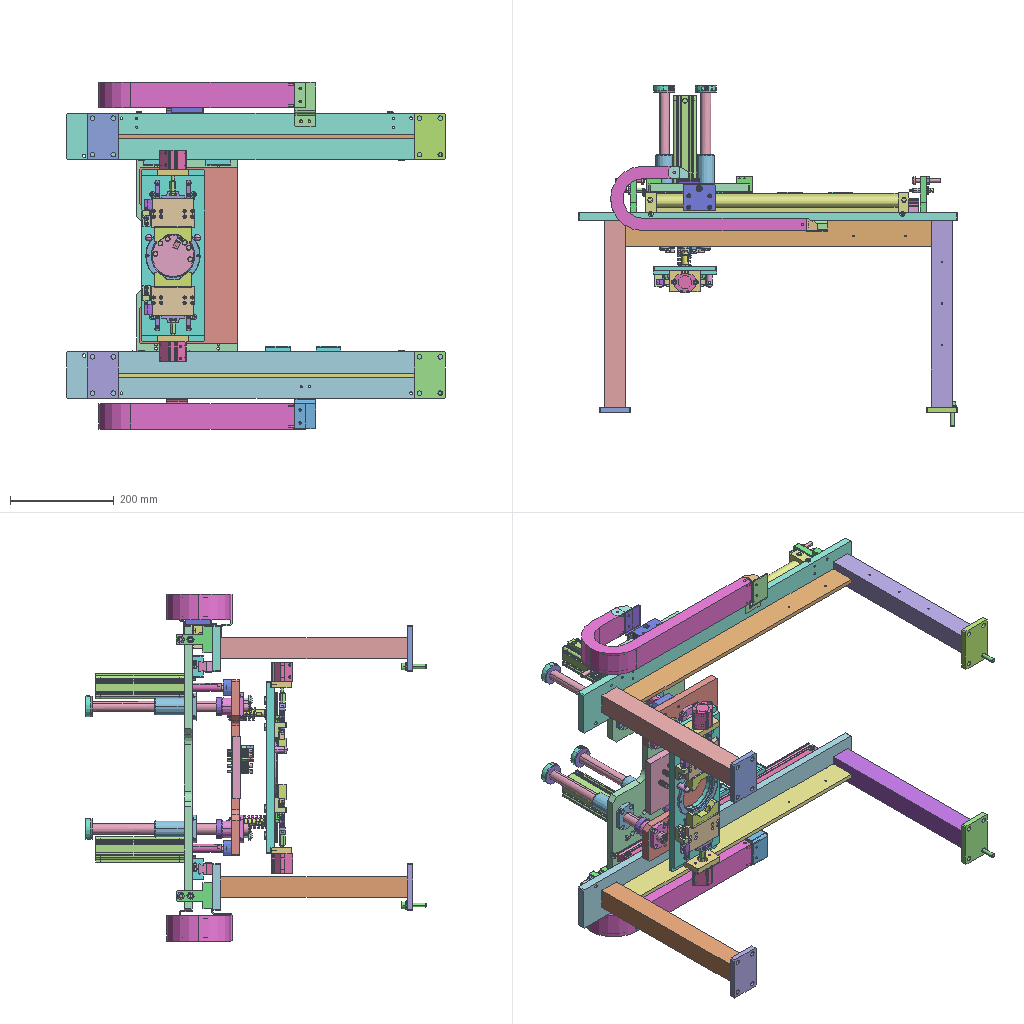Assembly | STEP file | 84 different items | 191 placed | box 730 x 656 x 669 mm
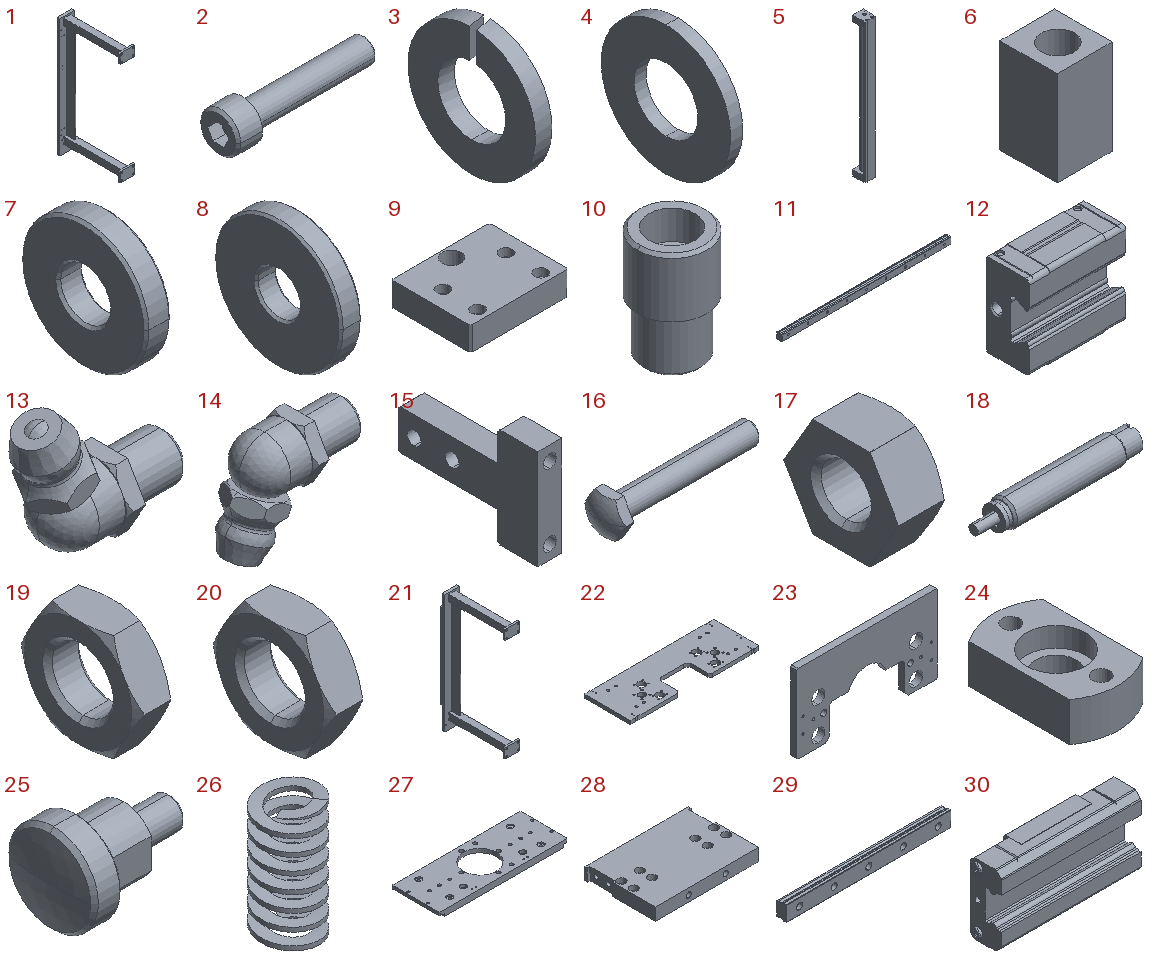Parts list (item | name | quantity | parent item | size | volume):
1 | 227H056235 BKT L_Default | x1 | in BKE LEFT ASSY_Default | 90 x 397 x 730 mm | 1763057 mm3
2 | CB8-40_Default | x2 | in CB8-40_SW8_W8_Default | 48 x 13 x 13 mm | 2919 mm3
3 | SW8_Default | x2 | in CB8-40_SW8_W8_Default | 2 x 15.4 x 15.396 mm | 260.908 mm3
4 | W8_Default | x2 | in CB8-40_SW8_W8_Default | 1.6 x 17 x 17 mm | 274.5 mm3
5 | 1_22 | x1 | in CY3R20-400_0_0_0_ | 38 x 45 x 507 mm | 342887 mm3
6 | 2_22 | x1 | in CY3R20-400_0_0_0_ | 36 x 37.5 x 62 mm | 60624 mm3
7 | wasmh10_4_2_2_03 | x2 | in BKE LEFT ASSY_Default | 2 x 10 x 10 mm | 130.188 mm3
8 | wasmh12_4_2_2_03 | x4 | in BKE LEFT ASSY_Default, BKE Right ASSY_Default | 2 x 12 x 12 mm | 199.051 mm3
9 | 227H056245 Move Block_Default | x1 | in BKE LEFT ASSY_Default | 62 x 50 x 15 mm | 43132 mm3
10 | 227H056246 Shaft_Default | x1 | in BKE LEFT ASSY_Default | 12 x 12 x 19 mm | 1355 mm3
11 | SSR20XV52020 Track | x2 | in SSR20XV2UU520200B047_700 | 520 x 15.5 x 20 mm | 137719 mm3
12 | SSR20XVUUB Slide15-25 | x4 | in SSR20XV2UU520200B047_700 | 47.7 x 22 x 42 mm | 34844 mm3
13 | SSR20XVUUBGNPJ-20-25 | x2 | in SSR20XV2UU520200B047_700 | 18.6 x 9.238 x 15.618 mm | 860 mm3
14 | SSR20XVUUBGNPJ2-20-25 | x2 | in SSR20XV2UU520200B047_700 | 18.6 x 9.238 x 15.618 mm | 860.005 mm3
15 | 227H056256 Stop Block_Default | x5 | in TRU, P_Default | 12 x 70 x 50 mm | 21777 mm3
16 | 1_12 | x5 | in stbb8_50_2_03 | - | 3160 mm3
17 | 2_12 | x5 | in stbb8_50_2_03 | 6.5 x 15 x 13 mm | 713.15 mm3
18 | Sceond1_16 | x5 | in SceondRB0806_0_ | 46.8 x 8 x 8 mm | 1959 mm3
19 | Sceond2_16 | x5 | in SceondRB0806_0_ | 4 x 13.856 x 12 mm | 338.014 mm3
20 | Sceond3_11 | x5 | in SceondRB0806_0_ | 4 x 13.856 x 12 mm | 338.014 mm3
21 | 227H056236 BKT R_Default | x1 | in BKE Right ASSY_Default | 90 x 397 x 730 mm | 1763979 mm3
22 | 227H056239 Base | x1 | in qnBANSONG_Default | 550 x 195 x 15 mm | 1337407 mm3
23 | 227H056238 Middle Base_Default | x1 | in qnBANSONG_Default | 340 x 15 x 190 mm | 662186 mm3
24 | qnSceondFJMC8part4 | x2 | in qnSceondFJMC8-00_FJMC8 | 30 x 51 x 16 mm | 15639 mm3
25 | qnSceondFJMC8part5 | x2 | in qnSceondFJMC8-00_FJMC8 | 32 x 23 x 23 mm | 5961 mm3
26 | SWY24.5-55_Default | x2 | in qnBANSONG_Default | 26.648 x 26.648 x 55 mm | 5041 mm3
27 | 227H056237 Under Base | x1 | in qnSceondMove 1_Default | 332 x 122 x 15 mm | 468693 mm3
28 | 227H056248 JIG Block | x2 | in qnSceondMove 1_Default | 84 x 57 x 10 mm | 44690 mm3
29 | 2SRS9MUU+95L | x4 | in 29 | 95 x 5.5 x 9 mm | 3697 mm3
30 | qnSceond_SRS9MQZUU Slider | x4 | in 29 | 40.8 x 9.1 x 20 mm | 5179 mm3
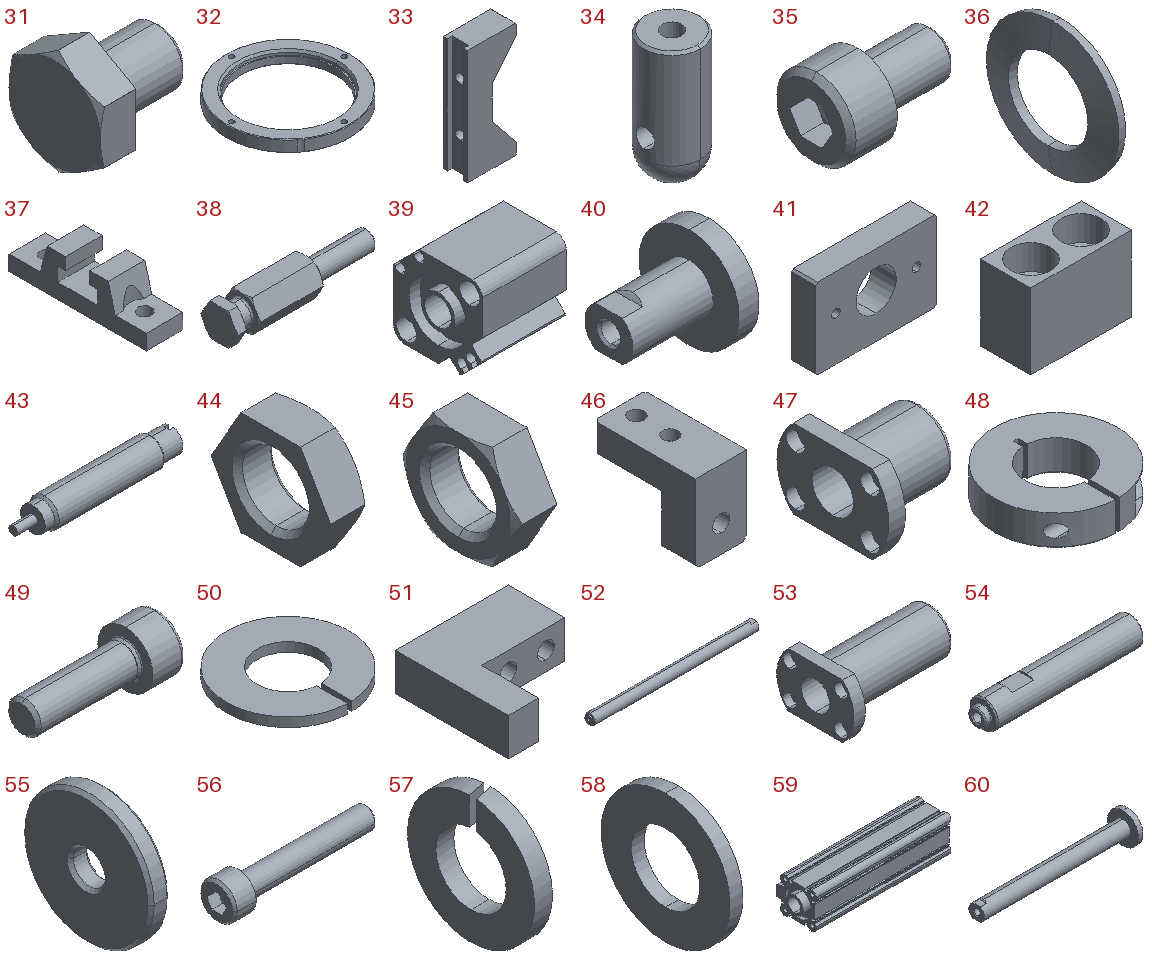31 | STEHN13 | x4 | in qnSceondMove 1_Default | 15 x 13 x 15 mm | 1216 mm3
32 | 227H056250 JIG_Default | x1 | in qnSceondMove 1_Default | 105 x 105 x 10 mm | 33679 mm3
33 | 227H056247 JIG_Default | x2 | in qnSceondMove 1_Default | 30 x 15 x 70 mm | 19012 mm3
34 | 227H056251 Pin_Default | x2 | in qnSceondMove 1_Default | 12 x 12 x 27 mm | 2502 mm3
35 | CB5-8_Default | x1 | in CB5-8_CW5_Default | 13 x 8.5 x 8.5 mm | 398.056 mm3
36 | CW5_Default | x1 | in CB5-8_CW5_Default | 0.85 x 9 x 9 mm | 22.263 mm3
37 | hlre7_2_03 | x2 | in qnSceondMove 1_Default | 12 x 45 x 13.5 mm | 3705 mm3
38 | fjdl6_1_0_4_20_2_03 | x2 | in qnSceondMove 1_Default | 46 x 11.547 x 10 mm | 2689 mm3
39 | 1_9 | x2 | in CDQ2B25-5DZ_0_0_0_ | 37.5 x 40 x 40 mm | 38658 mm3
40 | 2_9 | x2 | in CDQ2B25-5DZ_0_0_0_ | 25 x 25 x 25 mm | 4428 mm3
41 | 227H056249 Cylinder BKT_Default | x2 | in qnSceondMove 1_Default | 60 x 12 x 40 mm | 24374 mm3
42 | 227H056259 Stop Block_Default | x2 | in qnSceondMove 1_Default | 20 x 10 x 15 mm | 2179 mm3
43 | 1_10 | x2 | in RB0604_0_ | 32.5 x 6 x 6 mm | 755.606 mm3
44 | 2_10 | x2 | in RB0604_0_ | 3 x 9.238 x 8 mm | 99.469 mm3
45 | 3_1 | x2 | in RB0604_0_ | 3 x 9.238 x 8 mm | 99.469 mm3
46 | 227H056261 Stop Block_Default | x2 | in qnSceondMove 1_Default | 15 x 30 x 23 mm | 5038 mm3
47 | qnslhfc20_2_03 | x4 | in qnBANSONG_Default | 42 x 54 x 38 mm | 27385 mm3
48 | qnSceond1_10 | x4 | in qnSceondpscdj20_13_2_031 | 40 x 39.986 x 10 mm | 8415 mm3
49 | qnSceond2_10 | x4 | in qnSceondpscdj20_13_2_031 | 21 x 8.5 x 8.5 mm | 547.959 mm3
50 | qnSceond3_2 | x4 | in qnSceondpscdj20_13_2_031 | 40 x 39.986 x 3 mm | 2782 mm3
51 | 227H056244 Stopper_Default | x4 | in qnBANSONG_Default | 30 x 30 x 10 mm | 4879 mm3
52 | sfpg20_315_f3_p15_m6_sc305_2_03 | x4 | in qnBANSONG_Default | 318 x 20 x 20 mm | 98846 mm3
53 | lhfcwmf20_2_03 | x4 | in qnBANSONG_Default | 80 x 54 x 38 mm | 46009 mm3
54 | sfppa13_68_f3_p8_m5_n5_sc10_2_03 | x2 | in qnBANSONG_Default | 71 x 13 x 13 mm | 8114 mm3
55 | wssb20_5_3_2_03 | x2 | in qnBANSONG_Default | 3 x 20 x 20 mm | 863.938 mm3
56 | CB5-30_Default | x1 | in CB5-30_SW5_W5_Default | 35 x 8.5 x 8.5 mm | 830.025 mm3
57 | SW5_Default | x1 | in CB5-30_SW5_W5_Default | 1.3 x 9.2 x 9.198 mm | 58.481 mm3
58 | W5_Default | x1 | in CB5-30_SW5_W5_Default | 1 x 10 x 10 mm | 56.478 mm3
59 | 1 | x2 | in CDQ2A32-125DCZ | 175.5 x 49.5 x 45 mm | 171932 mm3
60 | 2 | x2 | in CDQ2A32-125DCZ | 157 x 32 x 32 mm | 34054 mm3
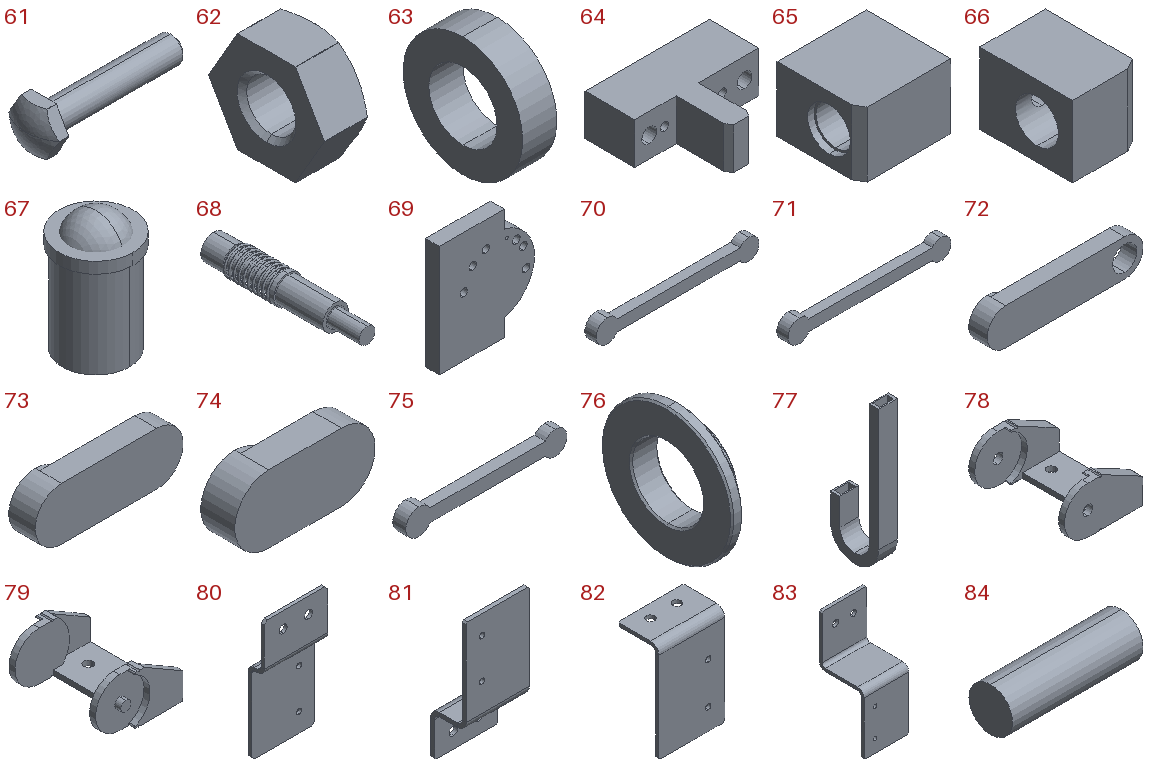61 | 1_5 | x2 | in stbb10_50_2_03 | - | 5335 mm3
62 | 2_5 | x2 | in stbb10_50_2_03 | 8 x 19.6 x 17 mm | 1538 mm3
63 | urws35_20_10_2_03 | x4 | in qnBANSONG_Default | 10 x 35 x 35 mm | 6480 mm3
64 | 22DDSceond144_Default | x1 | in 22DDSceondchatou_Default | 30 x 25 x 10 mm | 3740 mm3
65 | 22DDSceond4trr_Default | x1 | in 22DDSceondchatou_Default | 13.8 x 13 x 10 mm | 1356 mm3
66 | 22DDSceondwrwet_Default | x1 | in 22DDSceondchatou_Default | 9.2 x 13 x 10 mm | 888.519 mm3
67 | 22DDSceondZAL02-M6_Default | x2 | in 22DDSceondchatou_Default | 6.6 x 6.6 x 10.6 mm | 325.856 mm3
68 | 22CPMM160_Default | x6 | in 22DDSceoWWnd Terminal Inspection Tip sss_Default | 9.1 x 48.5 x 9.1 mm | 1897 mm3
69 | jjjj_Default | x1 | in 22DDSceoWWnd Terminal Inspection Tip sss_Default | 102.5 x 15 x 120 mm | 138148 mm3
70 | 222_Default | x1 | in 22DDSceoWWnd Terminal Inspection Tip sss_Default | 86.9 x 6 x 12 mm | 3087 mm3
71 | 333_Default | x1 | in 22DDSceoWWnd Terminal Inspection Tip sss_Default | 88.1 x 6 x 12 mm | 3123 mm3
72 | 444_Default | x1 | in 22DDSceoWWnd Terminal Inspection Tip sss_Default | 51 x 6 x 12 mm | 2767 mm3
73 | TYYUTI_Default | x1 | in 22DDSceoWWnd Terminal Inspection Tip sss_Default | 33.7 x 6 x 12 mm | 1981 mm3
74 | JTJTRUYIU_Default | x1 | in 22DDSceoWWnd Terminal Inspection Tip sss_Default | 24.8 x 6 x 12 mm | 1447 mm3
75 | 111_Default | x1 | in 22DDSceoWWnd Terminal Inspection Tip sss_Default | 75 x 6 x 12 mm | 2730 mm3
76 | ftcm_d16_5_h24_v13_0_t2_0_l5_0_2_03 | x4 | in qnBANSONG_Default | 5 x 24 x 24 mm | 869.825 mm3
77 | 18.37.38-18-18.37.12PZ_Default | x2 | in DFGG_Default | 49 x 124 x 377 mm | 276461 mm3
78 | 18_37_1 | x2 | in DFGG_Default | 40.3 x 49 x 24 mm | 8325 mm3
79 | 18_37_3 | x2 | in DFGG_Default | 40.3 x 49 x 24 mm | 7598 mm3
80 | 227H056252 BKT_Default | x1 | in 17 | 40 x 10 x 80 mm | 6705 mm3
81 | 227h056253 BKT_Default | x1 | in 17 | 40 x 22.5 x 85 mm | 9969 mm3
82 | 227H056254 BKT_Default | x1 | in 17 | 40 x 25 x 60 mm | 6386 mm3
83 | 227H056255 BKT_Default | x1 | in 17 | 40 x 40 x 96 mm | 12819 mm3
84 | HP5-15_Default | x4 | in 17 | 15 x 5 x 5 mm | 294.524 mm3
Placements (level | parent | child | x y z in mm | rotation matrix by rows):
1 | 17 | BKE LEFT ASSY_Default | 0.0 -0.0 230.0 | 1 0 0 0 1 0 0 0 1
2 | BKE LEFT ASSY_Default | 227H056235 BKT L_Default | -0.0 -0.0 -0.0 | 0 0 1 0 1 0 -1 0 0
2 | BKE LEFT ASSY_Default | CB8-40_SW8_W8_Default | 20.0 13.6 -35.0 | 0 1 0 -1 0 0 0 0 1
3 | CB8-40_SW8_W8_Default | CB8-40_Default | -0.0 -0.0 -0.0 | 1 0 0 0 1 0 0 0 1
3 | CB8-40_SW8_W8_Default | SW8_Default | 1.0 -0.0 -0.0 | 1 0 0 0 1 0 0 0 1
3 | CB8-40_SW8_W8_Default | W8_Default | 2.8 -0.0 -0.0 | 1 0 0 0 1 0 0 0 1
2 | BKE LEFT ASSY_Default | CY3R20-400_0_0_0_ | -84.5 481.55 68.762 | 0 0 1 1 0 0 0 1 -0
3 | CY3R20-400_0_0_0_ | 1_22 | -75.55 -42.762 -0.0 | 1 0 0 0 1 0 0 0 1
3 | CY3R20-400_0_0_0_ | 2_22 | -75.55 -42.762 -350.0 | 1 0 0 0 1 0 0 0 1
2 | BKE LEFT ASSY_Default | wasmh10_4_2_2_03 | -76.0 382.0 45.0 | 0 -0.9516 -0.3073 0 0.3073 -0.9516 1 0 0
2 | BKE LEFT ASSY_Default | wasmh10_4_2_2_03 | -561.0 382.0 45.0 | 0 -0.9516 -0.3073 0 0.3073 -0.9516 1 0 0
2 | BKE LEFT ASSY_Default | wasmh12_4_2_2_03 | -55.0 394.0 -45.0 | 0 0 1 0 1 0 -1 0 0
2 | BKE LEFT ASSY_Default | wasmh12_4_2_2_03 | -555.0 394.0 -45.0 | 0 0 1 0 1 0 -1 0 0
2 | BKE LEFT ASSY_Default | 227H056245 Move Block_Default | -467.5 414.5 46.0 | 1 0 0 0 1 0 0 0 1
2 | BKE LEFT ASSY_Default | 227H056246 Shaft_Default | -467.5 431.5 39.0 | 1 0 0 0 1 0 0 0 1
2 | BKE LEFT ASSY_Default | SSR20XV2UU520200B047_700 | -545.0 397.0 -35.0 | 1 0 0 0 1 0 0 0 1
3 | SSR20XV2UU520200B047_700 | SSR20XV52020 Track | -0.0 -0.0 -0.0 | 1 0 0 0 1 0 0 0 1
3 | SSR20XV2UU520200B047_700 | SSR20XVUUB Slide15-25 | 17.5 6.0 0.0 | 1 0 0 0 1 0 0 0 1
3 | SSR20XV2UU520200B047_700 | SSR20XVUUBGNPJ-20-25 | 3.85 6.0 -0.0 | 1 0 0 0 1 0 0 0 1
3 | SSR20XV2UU520200B047_700 | SSR20XVUUB Slide15-25 | 137.5 6.0 0.0 | 1 0 0 0 1 0 0 0 1
3 | SSR20XV2UU520200B047_700 | SSR20XVUUBGNPJ2-20-25 | 51.55 6.0 -0.0 | -1 0 0 0 1 0 0 0 -1
2 | BKE LEFT ASSY_Default | TRU;P_Default | -42.0 420.0 17.0 | 1 0 0 0 1 0 0 0 1
3 | TRU;P_Default | 227H056256 Stop Block_Default | -0.0 -0.0 -0.0 | 1 0 0 0 1 0 0 0 1
3 | TRU;P_Default | stbb8_50_2_03 | -9.75 27.0 -0.0 | 1 0 0 0 0.3709 -0.9287 0 0.9287 0.3709
4 | stbb8_50_2_03 | 1_12 | -0.0 -0.0 -0.0 | 1 0 0 0 1 0 0 0 1
4 | stbb8_50_2_03 | 2_12 | -0.0 -0.0 -0.0 | 1 0 0 0 1 0 0 0 1
3 | TRU;P_Default | SceondRB0806_0_ | -15.0 8.0 -0.0 | 1 0 0 0 0.9995 0.03109 0 -0.03109 0.9995
4 | SceondRB0806_0_ | Sceond1_16 | -0.0 -0.0 -0.0 | 1 0 0 0 1 0 0 0 1
4 | SceondRB0806_0_ | Sceond2_16 | -0.0 -0.0 -0.0 | 1 0 0 0 1 0 0 0 1
4 | SceondRB0806_0_ | Sceond3_11 | 4.733 -0.0 -0.0 | 1 0 0 0 1 0 0 0 1
2 | BKE LEFT ASSY_Default | TRU;P_Default | -588.0 420.0 17.0 | -1 0 0 0 1 0 0 0 -1
3 | TRU;P_Default | 227H056256 Stop Block_Default | -0.0 -0.0 -0.0 | 1 0 0 0 1 0 0 0 1
3 | TRU;P_Default | stbb8_50_2_03 | -9.75 27.0 -0.0 | 1 0 0 0 0.3709 -0.9287 0 0.9287 0.3709
4 | stbb8_50_2_03 | 1_12 | -0.0 -0.0 -0.0 | 1 0 0 0 1 0 0 0 1
4 | stbb8_50_2_03 | 2_12 | -0.0 -0.0 -0.0 | 1 0 0 0 1 0 0 0 1
3 | TRU;P_Default | SceondRB0806_0_ | -15.0 8.0 -0.0 | 1 0 0 0 0.9995 0.03109 0 -0.03109 0.9995
4 | SceondRB0806_0_ | Sceond1_16 | -0.0 -0.0 -0.0 | 1 0 0 0 1 0 0 0 1
4 | SceondRB0806_0_ | Sceond2_16 | -0.0 -0.0 -0.0 | 1 0 0 0 1 0 0 0 1
4 | SceondRB0806_0_ | Sceond3_11 | 4.733 -0.0 -0.0 | 1 0 0 0 1 0 0 0 1
1 | 17 | BKE Right ASSY_Default | -0.0 -0.0 -230.0 | 1 0 0 0 1 0 0 0 1
2 | BKE Right ASSY_Default | 227H056236 BKT R_Default | -0.0 -0.0 -0.0 | 0 0 1 0 1 0 -1 0 0
2 | BKE Right ASSY_Default | CB8-40_SW8_W8_Default | 20.0 13.6 -35.0 | 0 1 0 -1 0 0 0 0 1
3 | CB8-40_SW8_W8_Default | CB8-40_Default | -0.0 -0.0 -0.0 | 1 0 0 0 1 0 0 0 1
3 | CB8-40_SW8_W8_Default | SW8_Default | 1.0 -0.0 -0.0 | 1 0 0 0 1 0 0 0 1
3 | CB8-40_SW8_W8_Default | W8_Default | 2.8 -0.0 -0.0 | 1 0 0 0 1 0 0 0 1
2 | BKE Right ASSY_Default | wasmh12_4_2_2_03 | -555.0 394.0 45.0 | 0 -0.9985 0.05496 0 -0.05496 -0.9985 1 0 -0
2 | BKE Right ASSY_Default | wasmh12_4_2_2_03 | -55.0 394.0 47.0 | 0 0 1 0 1 0 -1 0 0
2 | BKE Right ASSY_Default | SSR20XV2UU520200B047_700 | -545.0 397.0 35.0 | 1 0 0 0 1 0 0 0 1
3 | SSR20XV2UU520200B047_700 | SSR20XV52020 Track | -0.0 -0.0 -0.0 | 1 0 0 0 1 0 0 0 1
3 | SSR20XV2UU520200B047_700 | SSR20XVUUB Slide15-25 | 252.546 6.0 -0.0 | 1 0 0 0 1 0 0 0 1
3 | SSR20XV2UU520200B047_700 | SSR20XVUUBGNPJ-20-25 | 3.85 6.0 -0.0 | 1 0 0 0 1 0 0 0 1
3 | SSR20XV2UU520200B047_700 | SSR20XVUUB Slide15-25 | 349.573 6.0 -0.0 | 1 0 0 0 1 0 0 0 1
3 | SSR20XV2UU520200B047_700 | SSR20XVUUBGNPJ2-20-25 | 51.55 6.0 -0.0 | -1 0 0 0 1 0 0 0 -1
2 | BKE Right ASSY_Default | TRU;P_Default | -588.0 420.0 -17.0 | -1 0 0 0 1 0 0 0 -1
3 | TRU;P_Default | 227H056256 Stop Block_Default | -0.0 -0.0 -0.0 | 1 0 0 0 1 0 0 0 1
3 | TRU;P_Default | stbb8_50_2_03 | -9.75 27.0 -0.0 | 1 0 0 0 0.3709 -0.9287 0 0.9287 0.3709
4 | stbb8_50_2_03 | 1_12 | -0.0 -0.0 -0.0 | 1 0 0 0 1 0 0 0 1
4 | stbb8_50_2_03 | 2_12 | -0.0 -0.0 -0.0 | 1 0 0 0 1 0 0 0 1
3 | TRU;P_Default | SceondRB0806_0_ | -15.0 8.0 -0.0 | 1 0 0 0 0.9995 0.03109 0 -0.03109 0.9995
4 | SceondRB0806_0_ | Sceond1_16 | -0.0 -0.0 -0.0 | 1 0 0 0 1 0 0 0 1
4 | SceondRB0806_0_ | Sceond2_16 | -0.0 -0.0 -0.0 | 1 0 0 0 1 0 0 0 1
4 | SceondRB0806_0_ | Sceond3_11 | 4.733 -0.0 -0.0 | 1 0 0 0 1 0 0 0 1
2 | BKE Right ASSY_Default | TRU;P_Default | -42.0 420.0 -17.0 | 1 0 0 0 1 0 0 0 1
3 | TRU;P_Default | 227H056256 Stop Block_Default | -0.0 -0.0 -0.0 | 1 0 0 0 1 0 0 0 1
3 | TRU;P_Default | stbb8_50_2_03 | -9.75 27.0 -0.0 | 1 0 0 0 0.3709 -0.9287 0 0.9287 0.3709
4 | stbb8_50_2_03 | 1_12 | -0.0 -0.0 -0.0 | 1 0 0 0 1 0 0 0 1
4 | stbb8_50_2_03 | 2_12 | -0.0 -0.0 -0.0 | 1 0 0 0 1 0 0 0 1
3 | TRU;P_Default | SceondRB0806_0_ | -15.0 8.0 -0.0 | 1 0 0 0 0.9995 0.03109 0 -0.03109 0.9995
4 | SceondRB0806_0_ | Sceond1_16 | -0.0 -0.0 -0.0 | 1 0 0 0 1 0 0 0 1
4 | SceondRB0806_0_ | Sceond2_16 | -0.0 -0.0 -0.0 | 1 0 0 0 1 0 0 0 1
4 | SceondRB0806_0_ | Sceond3_11 | 4.733 -0.0 -0.0 | 1 0 0 0 1 0 0 0 1
1 | 17 | qnBANSONG_Default | -460.0 425.0 -0.0 | 0 0 -1 0 1 0 1 0 0
2 | qnBANSONG_Default | 227H056239 Base | -0.0 -0.0 -0.0 | 1 0 0 0 0 1 0 -1 0
2 | qnBANSONG_Default | 227H056238 Middle Base_Default | 0.0 -90.985 5.0 | -1 0 0 0 1 0 0 0 -1
2 | qnBANSONG_Default | qnSceondFJMC8-00_FJMC8 | -155.0 -59.985 35.0 | 1 0 0 0 0 -1 0 1 -0
3 | qnSceondFJMC8-00_FJMC8 | qnSceondFJMC8part4 | 0.0 -0.0 -0.0 | 1 0 0 0 1 0 0 0 1
3 | qnSceondFJMC8-00_FJMC8 | qnSceondFJMC8part5 | 0.0 -0.0 8.0 | 0 0 1 0 1 0 -1 0 0
2 | qnBANSONG_Default | qnSceondFJMC8-00_FJMC8 | 155.0 -59.985 35.0 | 1 0 0 0 0 -1 0 1 -0
3 | qnSceondFJMC8-00_FJMC8 | qnSceondFJMC8part4 | 0.0 -0.0 -0.0 | 1 0 0 0 1 0 0 0 1
3 | qnSceondFJMC8-00_FJMC8 | qnSceondFJMC8part5 | 0.0 -0.0 8.0 | 0 0 1 0 1 0 -1 0 0
2 | qnBANSONG_Default | SWY24.5-55_Default | -104.767 -157.652 35.635 | -0.3446 -0.9387 0 0 0 1 -0.9387 0.3446 0
2 | qnBANSONG_Default | qnSceondMove 1_Default | -0.0 -158.985 35.0 | 1 0 0 0 1 0 0 0 1
3 | qnSceondMove 1_Default | 227H056237 Under Base | -0.0 -0.0 -0.0 | 1 0 0 0 0 1 0 -1 0
3 | qnSceondMove 1_Default | 227H056248 JIG Block | -70.5 -10.0 0.0 | 0 -1 0 0 0 -1 1 0 -0
3 | qnSceondMove 1_Default | 2SRS9MUU+95L | -137.5 -0.0 -30.0 | 1 0 0 0 -1 0 0 0 -1
4 | 2SRS9MUU+95L | 2SRS9MUU+95L | 0.0 0.0 -0.0 | 1 0 0 0 1 0 0 0 1
4 | 2SRS9MUU+95L | qnSceond_SRS9MQZUU Slider | 52.0 0.9 -0.0 | 1 0 0 0 1 0 0 0 1
3 | qnSceondMove 1_Default | 2SRS9MUU+95L | -137.5 -0.0 30.0 | 1 0 0 0 -1 0 0 0 -1
4 | 2SRS9MUU+95L | 2SRS9MUU+95L | 0.0 0.0 0.0 | 1 0 0 0 1 0 0 0 1
4 | 2SRS9MUU+95L | qnSceond_SRS9MQZUU Slider | 52.0 0.9 0.0 | 1 0 0 0 1 0 0 0 1
3 | qnSceondMove 1_Default | 2SRS9MUU+95L | 57.5 -0.0 -30.0 | 1 0 0 0 -1 0 0 0 -1
4 | 2SRS9MUU+95L | 2SRS9MUU+95L | -0.0 0.0 0.0 | 1 0 0 0 1 0 0 0 1
4 | 2SRS9MUU+95L | qnSceond_SRS9MQZUU Slider | 23.0 0.9 -0.0 | 1 0 0 0 1 0 0 0 1
3 | qnSceondMove 1_Default | 2SRS9MUU+95L | 57.5 -0.0 30.0 | 1 0 0 0 -1 0 0 0 -1
4 | 2SRS9MUU+95L | 2SRS9MUU+95L | -0.0 0.0 0.0 | 1 0 0 0 1 0 0 0 1
4 | 2SRS9MUU+95L | qnSceond_SRS9MQZUU Slider | 23.0 0.9 -0.0 | 1 0 0 0 1 0 0 0 1
3 | qnSceondMove 1_Default | 227H056248 JIG Block | 65.5 -10.0 -0.0 | 0 1 0 0 0 -1 -1 0 -0
3 | qnSceondMove 1_Default | STEHN13 | 78.0 15.0 -0.0 | 0 1 0 -1 0 0 0 0 1
3 | qnSceondMove 1_Default | STEHN13 | -78.0 15.0 -0.0 | 0 0.1705 -0.9854 -1 0 0 0 0.9854 0.1705
3 | qnSceondMove 1_Default | 227H056250 JIG_Default | -0.0 -5.0 -0.0 | -1 0 0 0 0 -1 0 -1 0
3 | qnSceondMove 1_Default | 227H056247 JIG_Default | -61.5 -22.5 0.0 | 1 0 0 0 1 0 0 0 1
3 | qnSceondMove 1_Default | 227H056247 JIG_Default | 56.5 -22.5 -0.0 | -1 0 0 0 1 0 0 0 -1
3 | qnSceondMove 1_Default | 227H056251 Pin_Default | 35.0 -25.0 47.0 | 1 0 0 0 0 1 0 -1 0
3 | qnSceondMove 1_Default | 227H056251 Pin_Default | 35.0 -25.0 -47.0 | 1 0 0 0 0 1 0 -1 0
3 | qnSceondMove 1_Default | CB5-8_CW5_Default | -55.157 -13.625 14.645 | -1 0 0 0 -0.8471 -0.5315 0 -0.5315 0.8471
4 | CB5-8_CW5_Default | CB5-8_Default | -3.507 0.9755 1.032 | 1 0 0 0 1 0 0 0 1
4 | CB5-8_CW5_Default | CW5_Default | -3.507 0.9755 1.032 | 1 0 0 0 1 0 0 0 1
3 | qnSceondMove 1_Default | hlre7_2_03 | -115.5 -15.0 0.0 | 0 0 -1 -1 0 0 0 1 0
3 | qnSceondMove 1_Default | fjdl6_1_0_4_20_2_03 | -122.0 -15.0 0.0 | -1 0 0 0 0.9893 -0.1461 0 -0.1461 -0.9893
3 | qnSceondMove 1_Default | CDQ2B25-5DZ_0_0_0_ | -166.0 -15.0 0.0 | -1 0 0 0 -0.7071 -0.7071 0 -0.7071 0.7071
4 | CDQ2B25-5DZ_0_0_0_ | 1_9 | -0.0 -0.0 -0.0 | 1 0 0 0 1 0 0 0 1
4 | CDQ2B25-5DZ_0_0_0_ | 2_9 | -0.0 0.0 0.0 | 1 0 0 0 0.5826 0.8128 0 -0.8128 0.5826
3 | qnSceondMove 1_Default | 227H056249 Cylinder BKT_Default | -154.0 -13.0 -0.0 | 0 -1 0 0 0 -1 1 0 0
3 | qnSceondMove 1_Default | hlre7_2_03 | 110.5 -15.0 0.0 | 0 0 1 1 0 0 0 1 0
3 | qnSceondMove 1_Default | 227H056249 Cylinder BKT_Default | 166.0 -13.0 -0.0 | 0 -1 0 0 0 -1 1 0 -0
3 | qnSceondMove 1_Default | CDQ2B25-5DZ_0_0_0_ | 166.0 -15.0 0.0 | 1 0 0 0 -0.7071 -0.7071 0 0.7071 -0.7071
4 | CDQ2B25-5DZ_0_0_0_ | 1_9 | -0.0 0.0 -0.0 | 1 0 0 0 1 0 0 0 1
4 | CDQ2B25-5DZ_0_0_0_ | 2_9 | -5.0 -0.0 0.0 | 1 0 0 0 0.5857 -0.8105 0 0.8105 0.5857
3 | qnSceondMove 1_Default | fjdl6_1_0_4_20_2_03 | 117.0 -15.0 0.0 | 1 0 0 0 0.7867 -0.6173 0 0.6173 0.7867
3 | qnSceondMove 1_Default | 227H056259 Stop Block_Default | -103.5 -20.0 47.5 | 1 0 0 0 1 0 0 0 1
3 | qnSceondMove 1_Default | 227H056259 Stop Block_Default | 98.5 -20.0 47.5 | 1 0 0 0 1 0 0 0 1
3 | qnSceondMove 1_Default | RB0604_0_ | -92.0 -15.0 51.5 | 1 0 0 0 1 0 0 0 1
4 | RB0604_0_ | 1_10 | 0.0 -0.0 -0.0 | 1 0 0 0 1 0 0 0 1
4 | RB0604_0_ | 2_10 | 0.0 -0.0 -0.0 | 1 0 0 0 1 0 0 0 1
4 | RB0604_0_ | 3_1 | 0.0 -0.0 -0.0 | 1 0 0 0 1 0 0 0 1
3 | qnSceondMove 1_Default | 227H056261 Stop Block_Default | -77.0 -8.0 44.0 | 0 1 0 0 0 1 1 0 0
3 | qnSceondMove 1_Default | 227H056261 Stop Block_Default | 77.0 -8.0 59.0 | 0 -1 0 0 0 1 -1 0 0
3 | qnSceondMove 1_Default | RB0604_0_ | 92.0 -15.0 51.5 | -1 0 0 0 -0.09795 0.9952 0 0.9952 0.09795
4 | RB0604_0_ | 1_10 | 0.0 -0.0 -0.0 | 1 0 0 0 1 0 0 0 1
4 | RB0604_0_ | 2_10 | 0.0 -0.0 -0.0 | 1 0 0 0 1 0 0 0 1
4 | RB0604_0_ | 3_1 | 0.0 -0.0 -0.0 | 1 0 0 0 1 0 0 0 1
3 | qnSceondMove 1_Default | STEHN13 | -130.0 15.0 0.0 | 0 0.1705 -0.9854 -1 0 0 0 0.9854 0.1705
3 | qnSceondMove 1_Default | STEHN13 | 130.0 15.0 0.0 | 0 0.1705 -0.9854 -1 0 0 0 0.9854 0.1705
2 | qnBANSONG_Default | qnslhfc20_2_03 | -118.0 -98.985 75.0 | 0 1 0 1 0 0 0 0 -1
2 | qnBANSONG_Default | qnslhfc20_2_03 | -118.0 -98.985 -5.0 | 0 1 0 1 0 0 0 0 -1
2 | qnBANSONG_Default | qnslhfc20_2_03 | 118.0 -98.985 -5.0 | 0 1 0 1 0 0 0 0 -1
2 | qnBANSONG_Default | qnslhfc20_2_03 | 118.0 -98.985 75.0 | 0 1 0 1 0 0 0 0 -1
2 | qnBANSONG_Default | qnSceondpscdj20_13_2_031 | -118.0 200.031 -5.0 | 0.7871 -0.6168 0 0 0 -1 0.6168 0.7871 -0
3 | qnSceondpscdj20_13_2_031 | qnSceond1_10 | -0.0 -0.0 -0.0 | 1 0 0 0 1 0 0 0 1
3 | qnSceondpscdj20_13_2_031 | qnSceond2_10 | -0.0 -0.0 -0.0 | 1 0 0 0 1 0 0 0 1
3 | qnSceondpscdj20_13_2_031 | qnSceond3_2 | -0.0 -0.0 -0.0 | 1 0 0 0 1 0 0 0 1
2 | qnBANSONG_Default | qnSceondpscdj20_13_2_031 | -118.0 200.031 75.0 | 0.9991 0.04303 0 0 0 -1 -0.04303 0.9991 -0
3 | qnSceondpscdj20_13_2_031 | qnSceond1_10 | -0.0 -0.0 -0.0 | 1 0 0 0 1 0 0 0 1
3 | qnSceondpscdj20_13_2_031 | qnSceond2_10 | -0.0 -0.0 -0.0 | 1 0 0 0 1 0 0 0 1
3 | qnSceondpscdj20_13_2_031 | qnSceond3_2 | -0.0 -0.0 -0.0 | 1 0 0 0 1 0 0 0 1
2 | qnBANSONG_Default | qnSceondpscdj20_13_2_031 | 118.0 200.031 75.0 | 0.9975 -0.07033 0 0 0 -1 0.07033 0.9975 -0
3 | qnSceondpscdj20_13_2_031 | qnSceond1_10 | -0.0 -0.0 -0.0 | 1 0 0 0 1 0 0 0 1
3 | qnSceondpscdj20_13_2_031 | qnSceond2_10 | -0.0 -0.0 -0.0 | 1 0 0 0 1 0 0 0 1
3 | qnSceondpscdj20_13_2_031 | qnSceond3_2 | -0.0 -0.0 -0.0 | 1 0 0 0 1 0 0 0 1
2 | qnBANSONG_Default | qnSceondpscdj20_13_2_031 | 118.0 200.031 -5.0 | 0.6155 -0.7881 0 0 0 -1 0.7881 0.6155 -0
3 | qnSceondpscdj20_13_2_031 | qnSceond1_10 | -0.0 -0.0 -0.0 | 1 0 0 0 1 0 0 0 1
3 | qnSceondpscdj20_13_2_031 | qnSceond2_10 | -0.0 -0.0 -0.0 | 1 0 0 0 1 0 0 0 1
3 | qnSceondpscdj20_13_2_031 | qnSceond3_2 | -0.0 -0.0 -0.0 | 1 0 0 0 1 0 0 0 1
2 | qnBANSONG_Default | 227H056244 Stopper_Default | -247.0 15.0 95.0 | 0 0 1 0 1 0 -1 0 0
2 | qnBANSONG_Default | 227H056244 Stopper_Default | -247.0 15.0 -80.0 | 0 0 -1 0 1 0 1 0 -0
2 | qnBANSONG_Default | 227H056244 Stopper_Default | 247.0 15.0 -80.0 | 0 0 -1 0 1 0 1 0 -0
2 | qnBANSONG_Default | 227H056244 Stopper_Default | 247.0 15.0 95.0 | 0 0 1 0 1 0 -1 0 0
2 | qnBANSONG_Default | sfpg20_315_f3_p15_m6_sc305_2_03 | -118.0 -109.969 75.0 | 0 -0.007247 1 1 0 0 0 1 0.007247
2 | qnBANSONG_Default | sfpg20_315_f3_p15_m6_sc305_2_03 | 118.0 -109.969 75.0 | 0 -0.7788 0.6273 1 0 0 0 0.6273 0.7788
2 | qnBANSONG_Default | sfpg20_315_f3_p15_m6_sc305_2_03 | 118.0 -109.969 -5.0 | 0 -0.9856 0.1689 1 0 0 0 0.1689 0.9856
2 | qnBANSONG_Default | sfpg20_315_f3_p15_m6_sc305_2_03 | -118.0 -109.969 -5.0 | 0 -0.7308 0.6826 1 0 0 0 0.6826 0.7308
2 | qnBANSONG_Default | lhfcwmf20_2_03 | -118.0 -8.0 75.0 | 0 -1 0 1 0 0 0 0 1
2 | qnBANSONG_Default | lhfcwmf20_2_03 | -118.0 -8.0 -5.0 | 0 -1 0 1 0 0 0 0 1
2 | qnBANSONG_Default | lhfcwmf20_2_03 | 118.0 -8.0 -5.0 | 0 -1 0 1 0 0 0 0 1
2 | qnBANSONG_Default | lhfcwmf20_2_03 | 118.0 -8.0 75.0 | 0 -1 0 1 0 0 0 0 1
2 | qnBANSONG_Default | sfppa13_68_f3_p8_m5_n5_sc10_2_03 | -105.0 -143.985 35.0 | 0 -0.9725 -0.2329 1 0 0 0 -0.2329 0.9725
2 | qnBANSONG_Default | sfppa13_68_f3_p8_m5_n5_sc10_2_03 | 105.0 -143.985 35.0 | 0 -0.9725 -0.2329 1 0 0 0 -0.2329 0.9725
2 | qnBANSONG_Default | SWY24.5-55_Default | 104.42 -138.172 35.347 | 0.8577 -0.5141 0 0 0 1 -0.5141 -0.8577 0
2 | qnBANSONG_Default | wssb20_5_3_2_03 | -105.0 -75.985 35.0 | 0 -1 0 1 0 0 0 0 1
2 | qnBANSONG_Default | wssb20_5_3_2_03 | 105.0 -75.985 35.0 | 0 -1 0 1 0 0 0 0 1
2 | qnBANSONG_Default | CB5-30_SW5_W5_Default | -105.0 -70.685 35.0 | 0 1 0 -1 0 0 0 0 1
3 | CB5-30_SW5_W5_Default | CB5-30_Default | 0.0 0.0 -0.0 | 1 0 0 0 1 0 0 0 1
3 | CB5-30_SW5_W5_Default | SW5_Default | 0.65 -0.0 -0.0 | 1 0 0 0 1 0 0 0 1
3 | CB5-30_SW5_W5_Default | W5_Default | 1.8 -0.0 0.0 | 1 0 0 0 1 0 0 0 1
2 | qnBANSONG_Default | CDQ2A32-125DCZ | -155.0 15.0 35.0 | 0 -1 0 1 0 0 0 0 1
3 | CDQ2A32-125DCZ | 1 | -0.0 -0.0 -0.0 | 1 0 0 0 1 0 0 0 1
3 | CDQ2A32-125DCZ | 2 | -53.985 -0.0 -0.0 | 1 0 0 0 0.9409 -0.3386 0 0.3386 0.9409
2 | qnBANSONG_Default | CDQ2A32-125DCZ | 155.0 15.0 35.0 | 0 1 0 1 0 0 0 0 -1
3 | CDQ2A32-125DCZ | 1 | 0.0 -0.0 -0.0 | 1 0 0 0 1 0 0 0 1
3 | CDQ2A32-125DCZ | 2 | -53.985 -0.0 0.0 | 1 0 0 0 0.7786 -0.6275 0 0.6275 0.7786
2 | qnBANSONG_Default | stbb10_50_2_03 | 130.0 -108.985 35.0 | 0 -1 0 1 0 0 0 0 1
3 | stbb10_50_2_03 | 1_5 | 0.0 0.0 -0.0 | 1 0 0 0 1 0 0 0 1
3 | stbb10_50_2_03 | 2_5 | -11.0 0.0 -0.0 | 1 0 0 0 1 0 0 0 1
2 | qnBANSONG_Default | stbb10_50_2_03 | -130.0 -108.985 35.0 | 0 -1 0 1 0 0 0 0 1
3 | stbb10_50_2_03 | 1_5 | 0.0 0.0 -0.0 | 1 0 0 0 1 0 0 0 1
3 | stbb10_50_2_03 | 2_5 | -11.0 0.0 -0.0 | 1 0 0 0 1 0 0 0 1
2 | qnBANSONG_Default | urws35_20_10_2_03 | 118.0 -56.985 -5.0 | 0 0.427 0.9043 1 0 0 0 0.9043 -0.427
2 | qnBANSONG_Default | urws35_20_10_2_03 | 118.0 -56.985 75.0 | 0 0.427 0.9043 1 0 0 0 0.9043 -0.427
2 | qnBANSONG_Default | urws35_20_10_2_03 | -118.0 -56.985 -5.0 | 0 0.427 0.9043 1 0 0 0 0.9043 -0.427
2 | qnBANSONG_Default | urws35_20_10_2_03 | -118.0 -56.985 75.0 | 0 0.427 0.9043 1 0 0 0 0.9043 -0.427
2 | qnBANSONG_Default | 22DDSceoWWnd Terminal Inspection Tip sss_Default | -0.0 -78.037 35.0 | 0 0 1 0 1 0 -1 0 -0
3 | 22DDSceoWWnd Terminal Inspection Tip sss_Default | 22DDSceondchatou_Default | -11.711 -61.586 75.411 | -0.4602 0 0.8878 0 1 0 -0.8878 0 -0.4602
4 | 22DDSceondchatou_Default | 22DDSceond144_Default | 29.685 46.586 41.842 | 1 0 0 0 1 0 0 0 1
4 | 22DDSceondchatou_Default | 22DDSceond4trr_Default | 40.085 28.086 36.842 | 1 0 0 0 1 0 0 0 1
4 | 22DDSceondchatou_Default | 22DDSceondwrwet_Default | 21.585 28.086 36.842 | 1 0 0 0 1 0 0 0 1
4 | 22DDSceondchatou_Default | 22DDSceondZAL02-M6_Default | 26.185 26.586 41.842 | 0 0 1 0.287 0.9579 0 -0.9579 0.287 0
4 | 22DDSceondchatou_Default | 22DDSceondZAL02-M6_Default | 33.185 26.586 41.842 | 0 0 -1 0.8197 0.5727 0 0.5727 -0.8197 -0
3 | 22DDSceoWWnd Terminal Inspection Tip sss_Default | 22CPMM160_Default | -33.753 13.0 3.833 | -0.9411 0 -0.3382 0 -1 0 -0.3382 0 0.9411
3 | 22DDSceoWWnd Terminal Inspection Tip sss_Default | 22CPMM160_Default | -24.208 13.0 23.808 | -0.01742 0 -0.9998 0 -1 0 -0.9998 0 0.01742
3 | 22DDSceoWWnd Terminal Inspection Tip sss_Default | 22CPMM160_Default | -9.892 13.0 32.483 | 0.2832 0 0.959 0 -1 0 0.959 0 -0.2832
3 | 22DDSceoWWnd Terminal Inspection Tip sss_Default | 22CPMM160_Default | 23.013 13.0 25.012 | 0.2832 0 0.959 0 -1 0 0.959 0 -0.2832
3 | 22DDSceoWWnd Terminal Inspection Tip sss_Default | 22CPMM160_Default | 30.464 13.0 15.11 | 0.4722 0 0.8815 0 -1 0 0.8815 0 -0.4722
3 | 22DDSceoWWnd Terminal Inspection Tip sss_Default | 22CPMM160_Default | 33.338 13.0 -6.841 | 0.2832 0 0.959 0 -1 0 0.959 0 -0.2832
3 | 22DDSceoWWnd Terminal Inspection Tip sss_Default | jjjj_Default | -0.0 -0.0 0.0 | 1 0 0 0 1 0 0 0 1
3 | 22DDSceoWWnd Terminal Inspection Tip sss_Default | 222_Default | 0.217 -5.0 -7.456 | 0.8015 0 -0.598 0 1 0 0.598 0 0.8015
3 | 22DDSceoWWnd Terminal Inspection Tip sss_Default | 333_Default | 1.651 -5.0 -28.433 | 0.8264 0 -0.5631 0 1 0 0.5631 0 0.8264
3 | 22DDSceoWWnd Terminal Inspection Tip sss_Default | 444_Default | -27.341 -5.0 41.189 | 0.8948 0 0.4465 0 1 0 -0.4465 0 0.8948
3 | 22DDSceoWWnd Terminal Inspection Tip sss_Default | TYYUTI_Default | -34.607 -5.0 26.905 | 0.9584 0 0.2854 0 1 0 -0.2854 0 0.9584
3 | 22DDSceoWWnd Terminal Inspection Tip sss_Default | JTJTRUYIU_Default | -39.365 -5.0 6.91 | 0.8768 0 0.4808 0 1 0 -0.4808 0 0.8768
3 | 22DDSceoWWnd Terminal Inspection Tip sss_Default | 111_Default | -3.48 -5.0 7.514 | 0.8344 0 -0.5511 0 1 0 0.5511 0 0.8344
2 | qnBANSONG_Default | ftcm_d16_5_h24_v13_0_t2_0_l5_0_2_03 | -105.0 -143.985 35.0 | 0 -1 0 1 0 0 0 0 1
2 | qnBANSONG_Default | ftcm_d16_5_h24_v13_0_t2_0_l5_0_2_03 | 105.0 -143.985 35.0 | 0 -1 0 1 0 0 0 0 1
2 | qnBANSONG_Default | ftcm_d16_5_h24_v13_0_t2_0_l5_0_2_03 | -105.0 -90.985 35.0 | 0 -0.3363 -0.9418 -1 0 0 0 0.9418 -0.3363
2 | qnBANSONG_Default | ftcm_d16_5_h24_v13_0_t2_0_l5_0_2_03 | 105.0 -90.985 35.0 | 0 -0.4889 -0.8723 -1 0 0 0 0.8723 -0.4889
1 | 17 | TRU;P_Default | -42.0 420.0 247.0 | 1 0 0 0 1 0 0 0 1
2 | TRU;P_Default | 227H056256 Stop Block_Default | -0.0 -0.0 -0.0 | 1 0 0 0 1 0 0 0 1
2 | TRU;P_Default | stbb8_50_2_03 | -9.75 27.0 -0.0 | 1 0 0 0 0.3709 -0.9287 0 0.9287 0.3709
3 | stbb8_50_2_03 | 1_12 | -0.0 -0.0 -0.0 | 1 0 0 0 1 0 0 0 1
3 | stbb8_50_2_03 | 2_12 | -0.0 -0.0 -0.0 | 1 0 0 0 1 0 0 0 1
2 | TRU;P_Default | SceondRB0806_0_ | -15.0 8.0 -0.0 | 1 0 0 0 0.9995 0.03109 0 -0.03109 0.9995
3 | SceondRB0806_0_ | Sceond1_16 | -0.0 -0.0 -0.0 | 1 0 0 0 1 0 0 0 1
3 | SceondRB0806_0_ | Sceond2_16 | -0.0 -0.0 -0.0 | 1 0 0 0 1 0 0 0 1
3 | SceondRB0806_0_ | Sceond3_11 | 4.733 -0.0 -0.0 | 1 0 0 0 1 0 0 0 1
1 | 17 | DFGG_Default | -261.3 362.0 -309.5 | 0 0 1 0 1 0 -1 0 -0
2 | DFGG_Default | 18.37.38-18-18.37.12PZ_Default | -0.0 -0.0 -0.0 | 1 0 0 0 1 0 0 0 1
2 | DFGG_Default | 18_37_1 | -0.0 100.0 -254.3 | 0 1 0 0 0 1 1 0 -0
2 | DFGG_Default | 18_37_3 | 0.0 -0.0 -7.0 | 0 1 0 0 0 1 1 0 0
1 | 17 | DFGG_Default | -261.3 362.0 309.5 | 0 0 1 0 1 0 -1 0 0
2 | DFGG_Default | 18.37.38-18-18.37.12PZ_Default | -0.0 -0.0 -0.0 | 1 0 0 0 1 0 0 0 1
2 | DFGG_Default | 18_37_1 | -0.0 100.0 -254.3 | 0 1 0 0 0 1 1 0 -0
2 | DFGG_Default | 18_37_3 | 0.0 -0.0 -7.0 | 0 1 0 0 0 1 1 0 0
1 | 17 | 227H056252 BKT_Default | -467.3 440.0 284.0 | -1 0 0 0 1 0 0 0 -1
1 | 17 | 227h056253 BKT_Default | -260.0 347.5 274.0 | 1 0 0 0 1 0 0 0 1
1 | 17 | 227H056254 BKT_Default | -467.3 450.0 -275.0 | -1 0 0 0 -1 0 0 0 1
1 | 17 | 227H056255 BKT_Default | -260.0 350.0 -282.5 | 1 0 0 0 1 0 0 0 1
1 | 17 | HP5-15_Default | -407.5 433.0 171.5 | 0 0.4919 -0.8706 -1 0 0 0 0.8706 0.4919
1 | 17 | HP5-15_Default | -527.5 433.0 171.5 | 0 0.4919 -0.8706 -1 0 0 0 0.8706 0.4919
1 | 17 | HP5-15_Default | -527.5 433.0 -171.5 | 0 0.4919 -0.8706 -1 0 0 0 0.8706 0.4919
1 | 17 | HP5-15_Default | -407.5 433.0 -171.5 | 0 0.4919 -0.8706 -1 0 0 0 0.8706 0.4919